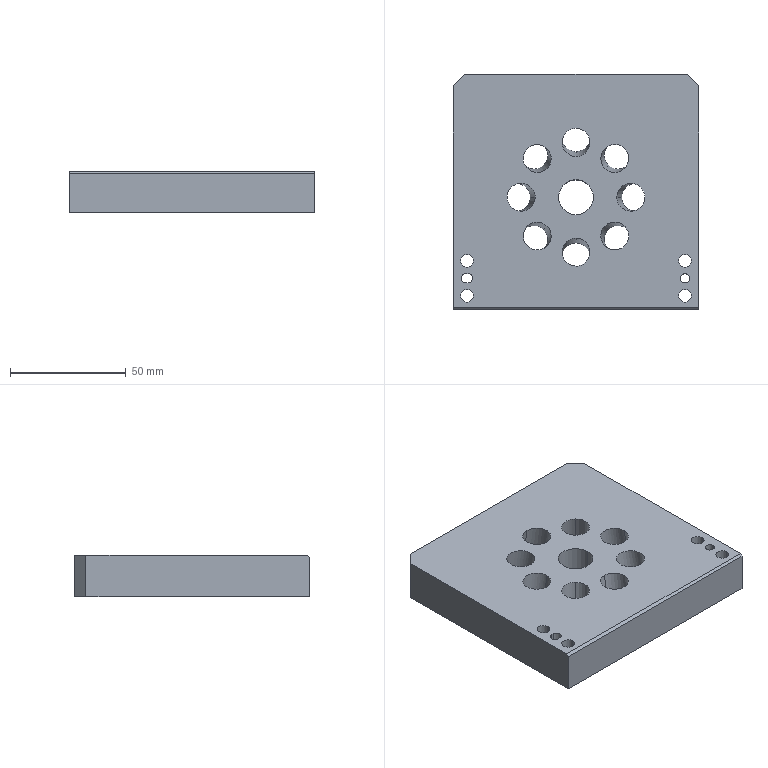Part | SolidWorks | features HoleWzd 3, Chamfer 2, CirPattern 1, Cut 1, Extrusion 1, ICE 1, RevCut 1 | 1 solid | 118 faces | box 106 x 101.44 x 18 mm | volume 167482 mm3 | cylinder 75 | plane 23 | cone 20 | commonest cylinder face diameters 2.5 x16 12 x16 16 x16 5.5 x8 9.5 x8 4 x5